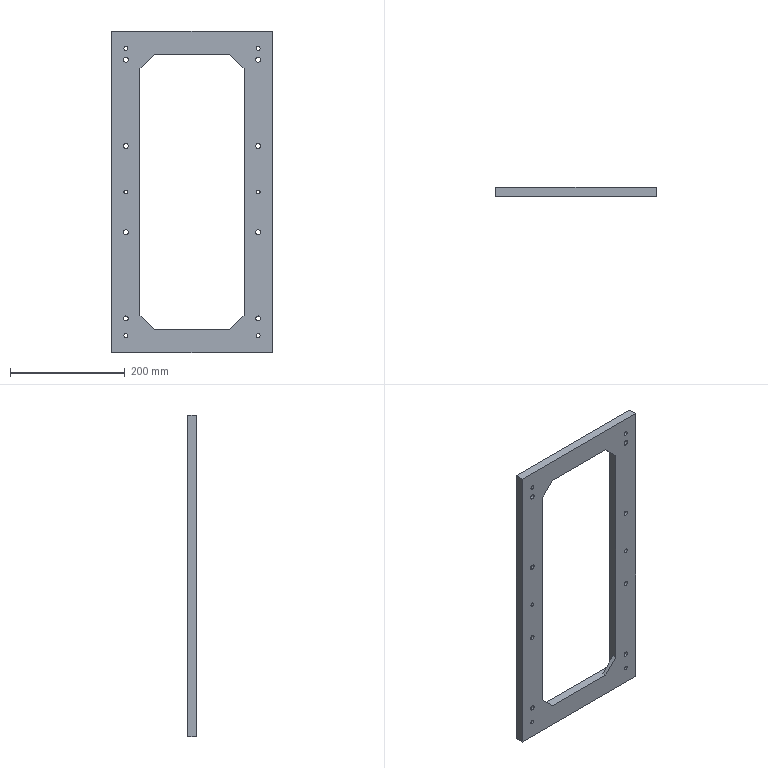Part | STEP file | A14-007 | 1 solid | 81 faces | box 280 x 15 x 560 mm | volume 1039428 mm3 | cylinder 51 | plane 28 | cone 2 | commonest cylinder face diameters 8.5 x16 13.5 x16 6.8 x12 20 x7